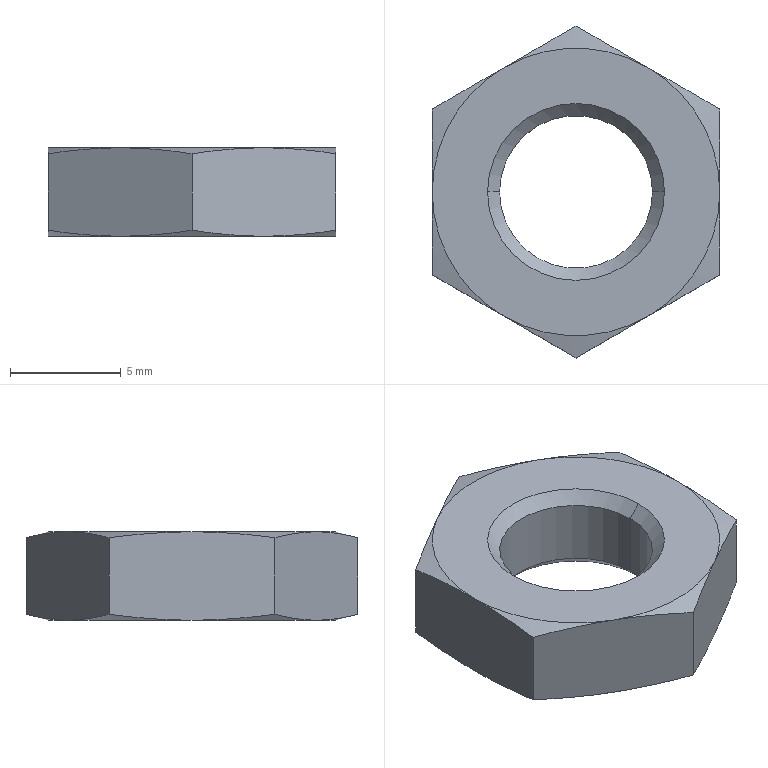Part | STEP file | _PSAM8screw_default | 1 solid | 26 faces | box 13 x 15.011 x 4 mm | volume 426.143 mm3 | cone 16 | plane 8 | cylinder 2 | commonest cylinder face diameters 6.917 x2